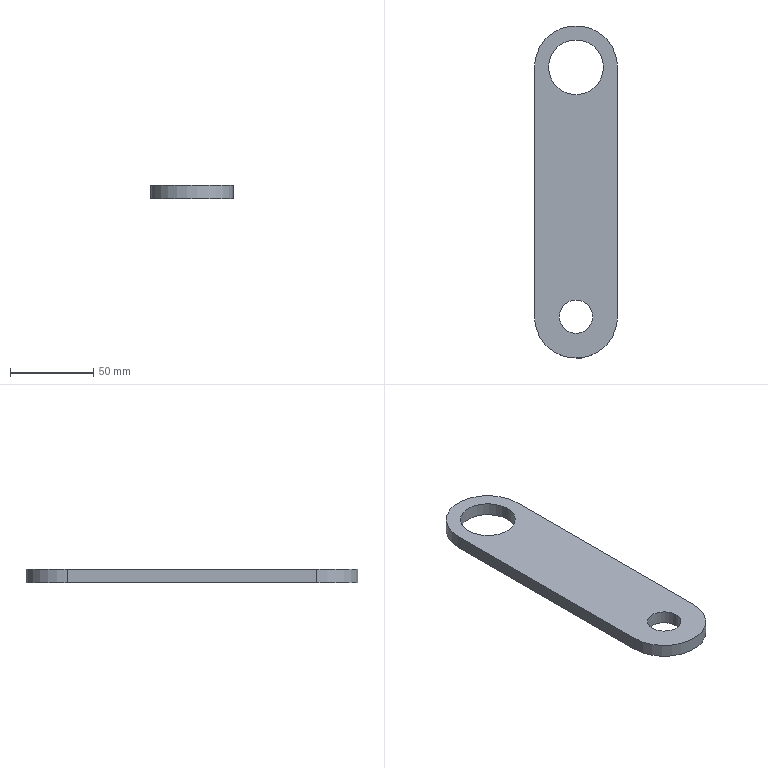Part | STEP file | 1 solid | 10 faces | box 50 x 200 x 8 mm | volume 66352 mm3 | cylinder 6 | plane 4 | commonest cylinder face diameters 20 x2 33 x2 50 x2
STEP:
#1=CARTESIAN_POINT('',(0.,0.,0.));
#2=DIRECTION('',(0.,0.,1.));
#3=DIRECTION('',(1.,0.,0.));
#4=AXIS2_PLACEMENT_3D('',#1,#2,#3);
#5=CARTESIAN_POINT('',(10.,-150.,-4.));
#6=VERTEX_POINT('',#5);
#7=CARTESIAN_POINT('',(-10.,-150.,-4.));
#8=VERTEX_POINT('',#7);
#9=CARTESIAN_POINT('',(0.,-150.,-4.));
#10=DIRECTION('',(0.,0.,1.));
#11=DIRECTION('',(1.,0.,0.));
#12=AXIS2_PLACEMENT_3D('',#9,#10,#11);
#13=CIRCLE('',#12,10.);
#14=CARTESIAN_POINT('',(0.,-150.,4.));
#15=DIRECTION('',(0.,0.,-1.));
#16=DIRECTION('',(-1.,0.,0.));
#17=AXIS2_PLACEMENT_3D('',#14,#15,#16);
#18=CYLINDRICAL_SURFACE('',#17,10.);
#19=CARTESIAN_POINT('',(3.142,8.));
#20=DIRECTION('',(-1.,0.));
#21=VECTOR('',#20,1.);
#22=LINE('',#19,#21);
#23=(GEOMETRIC_REPRESENTATION_CONTEXT(2)PARAMETRIC_REPRESENTATION_CONTEXT()REPRESENTATION_CONTEXT('',''));
#24=DEFINITIONAL_REPRESENTATION('',(#22),#23);
#25=PCURVE('',#18,#24);
#26=CARTESIAN_POINT('',(0.,0.,-4.));
#27=DIRECTION('',(0.,0.,1.));
#28=DIRECTION('',(1.,0.,0.));
#29=AXIS2_PLACEMENT_3D('',#26,#27,#28);
#30=PLANE('',#29);
#31=CARTESIAN_POINT('',(0.,-150.));
#32=DIRECTION('',(1.,0.));
#33=AXIS2_PLACEMENT_2D('',#31,#32);
#34=CIRCLE('',#33,10.);
#35=(GEOMETRIC_REPRESENTATION_CONTEXT(2)PARAMETRIC_REPRESENTATION_CONTEXT()REPRESENTATION_CONTEXT('',''));
#36=DEFINITIONAL_REPRESENTATION('',(#34),#35);
#37=PCURVE('',#30,#36);
#38=SURFACE_CURVE('',#13,(#25,#37),.PCURVE_S1.);
#39=EDGE_CURVE('',#6,#8,#38,.T.);
#40=ORIENTED_EDGE('',*,*,#39,.T.);
#41=CARTESIAN_POINT('',(-10.,-150.,4.));
#42=VERTEX_POINT('',#41);
#43=CARTESIAN_POINT('',(-10.,-150.,4.));
#44=DIRECTION('',(0.,0.,-1.));
#45=VECTOR('',#44,1.);
#46=LINE('',#43,#45);
#47=CARTESIAN_POINT('',(0.,0.));
#48=DIRECTION('',(0.,1.));
#49=VECTOR('',#48,1.);
#50=LINE('',#47,#49);
#51=(GEOMETRIC_REPRESENTATION_CONTEXT(2)PARAMETRIC_REPRESENTATION_CONTEXT()REPRESENTATION_CONTEXT('',''));
#52=DEFINITIONAL_REPRESENTATION('',(#50),#51);
#53=PCURVE('',#18,#52);
#54=CARTESIAN_POINT('',(0.,-150.,4.));
#55=DIRECTION('',(0.,0.,-1.));
#56=DIRECTION('',(-1.,0.,0.));
#57=AXIS2_PLACEMENT_3D('',#54,#55,#56);
#58=CYLINDRICAL_SURFACE('',#57,10.);
#59=CARTESIAN_POINT('',(6.283,0.));
#60=DIRECTION('',(0.,1.));
#61=VECTOR('',#60,1.);
#62=LINE('',#59,#61);
#63=(GEOMETRIC_REPRESENTATION_CONTEXT(2)PARAMETRIC_REPRESENTATION_CONTEXT()REPRESENTATION_CONTEXT('',''));
#64=DEFINITIONAL_REPRESENTATION('',(#62),#63);
#65=PCURVE('',#58,#64);
#66=SURFACE_CURVE('',#46,(#53,#65),.PCURVE_S1.);
#67=EDGE_CURVE('',#42,#8,#66,.T.);
#68=ORIENTED_EDGE('',*,*,#67,.F.);
#69=CARTESIAN_POINT('',(10.,-150.,4.));
#70=VERTEX_POINT('',#69);
#71=CARTESIAN_POINT('',(0.,-150.,4.));
#72=DIRECTION('',(0.,0.,1.));
#73=DIRECTION('',(1.,0.,0.));
#74=AXIS2_PLACEMENT_3D('',#71,#72,#73);
#75=CIRCLE('',#74,10.);
#76=CARTESIAN_POINT('',(3.142,0.));
#77=DIRECTION('',(-1.,0.));
#78=VECTOR('',#77,1.);
#79=LINE('',#76,#78);
#80=(GEOMETRIC_REPRESENTATION_CONTEXT(2)PARAMETRIC_REPRESENTATION_CONTEXT()REPRESENTATION_CONTEXT('',''));
#81=DEFINITIONAL_REPRESENTATION('',(#79),#80);
#82=PCURVE('',#18,#81);
#83=CARTESIAN_POINT('',(0.,0.,4.));
#84=DIRECTION('',(0.,0.,1.));
#85=DIRECTION('',(1.,0.,0.));
#86=AXIS2_PLACEMENT_3D('',#83,#84,#85);
#87=PLANE('',#86);
#88=CARTESIAN_POINT('',(0.,-150.));
#89=DIRECTION('',(1.,0.));
#90=AXIS2_PLACEMENT_2D('',#88,#89);
#91=CIRCLE('',#90,10.);
#92=(GEOMETRIC_REPRESENTATION_CONTEXT(2)PARAMETRIC_REPRESENTATION_CONTEXT()REPRESENTATION_CONTEXT('',''));
#93=DEFINITIONAL_REPRESENTATION('',(#91),#92);
#94=PCURVE('',#87,#93);
#95=SURFACE_CURVE('',#75,(#82,#94),.PCURVE_S1.);
#96=EDGE_CURVE('',#70,#42,#95,.T.);
#97=ORIENTED_EDGE('',*,*,#96,.F.);
#98=CARTESIAN_POINT('',(10.,-150.,4.));
#99=DIRECTION('',(0.,0.,-1.));
#100=VECTOR('',#99,1.);
#101=LINE('',#98,#100);
#102=CARTESIAN_POINT('',(3.142,0.));
#103=DIRECTION('',(0.,1.));
#104=VECTOR('',#103,1.);
#105=LINE('',#102,#104);
#106=(GEOMETRIC_REPRESENTATION_CONTEXT(2)PARAMETRIC_REPRESENTATION_CONTEXT()REPRESENTATION_CONTEXT('',''));
#107=DEFINITIONAL_REPRESENTATION('',(#105),#106);
#108=PCURVE('',#18,#107);
#109=CARTESIAN_POINT('',(3.142,0.));
#110=DIRECTION('',(0.,1.));
#111=VECTOR('',#110,1.);
#112=LINE('',#109,#111);
#113=(GEOMETRIC_REPRESENTATION_CONTEXT(2)PARAMETRIC_REPRESENTATION_CONTEXT()REPRESENTATION_CONTEXT('',''));
#114=DEFINITIONAL_REPRESENTATION('',(#112),#113);
#115=PCURVE('',#58,#114);
#116=SURFACE_CURVE('',#101,(#108,#115),.PCURVE_S1.);
#117=EDGE_CURVE('',#70,#6,#116,.T.);
#118=ORIENTED_EDGE('',*,*,#117,.T.);
#119=EDGE_LOOP('',(#40,#68,#97,#118));
#120=FACE_BOUND('',#119,.F.);
#121=ADVANCED_FACE('',(#120),#18,.F.);
#122=CARTESIAN_POINT('',(16.5,0.,-4.));
#123=VERTEX_POINT('',#122);
#124=CARTESIAN_POINT('',(-16.5,0.,-4.));
#125=VERTEX_POINT('',#124);
#126=CARTESIAN_POINT('',(0.,0.,-4.));
#127=DIRECTION('',(0.,0.,1.));
#128=DIRECTION('',(1.,0.,0.));
#129=AXIS2_PLACEMENT_3D('',#126,#127,#128);
#130=CIRCLE('',#129,16.5);
#131=CARTESIAN_POINT('',(0.,0.,4.));
#132=DIRECTION('',(0.,0.,-1.));
#133=DIRECTION('',(-1.,0.,0.));
#134=AXIS2_PLACEMENT_3D('',#131,#132,#133);
#135=CYLINDRICAL_SURFACE('',#134,16.5);
#136=CARTESIAN_POINT('',(3.142,8.));
#137=DIRECTION('',(-1.,0.));
#138=VECTOR('',#137,1.);
#139=LINE('',#136,#138);
#140=(GEOMETRIC_REPRESENTATION_CONTEXT(2)PARAMETRIC_REPRESENTATION_CONTEXT()REPRESENTATION_CONTEXT('',''));
#141=DEFINITIONAL_REPRESENTATION('',(#139),#140);
#142=PCURVE('',#135,#141);
#143=CARTESIAN_POINT('',(0.,0.));
#144=DIRECTION('',(1.,0.));
#145=AXIS2_PLACEMENT_2D('',#143,#144);
#146=CIRCLE('',#145,16.5);
#147=(GEOMETRIC_REPRESENTATION_CONTEXT(2)PARAMETRIC_REPRESENTATION_CONTEXT()REPRESENTATION_CONTEXT('',''));
#148=DEFINITIONAL_REPRESENTATION('',(#146),#147);
#149=PCURVE('',#30,#148);
#150=SURFACE_CURVE('',#130,(#142,#149),.PCURVE_S1.);
#151=EDGE_CURVE('',#123,#125,#150,.T.);
#152=ORIENTED_EDGE('',*,*,#151,.T.);
#153=CARTESIAN_POINT('',(-16.5,0.,4.));
#154=VERTEX_POINT('',#153);
#155=CARTESIAN_POINT('',(-16.5,0.,4.));
#156=DIRECTION('',(0.,0.,-1.));
#157=VECTOR('',#156,1.);
#158=LINE('',#155,#157);
#159=CARTESIAN_POINT('',(0.,0.));
#160=DIRECTION('',(0.,1.));
#161=VECTOR('',#160,1.);
#162=LINE('',#159,#161);
#163=(GEOMETRIC_REPRESENTATION_CONTEXT(2)PARAMETRIC_REPRESENTATION_CONTEXT()REPRESENTATION_CONTEXT('',''));
#164=DEFINITIONAL_REPRESENTATION('',(#162),#163);
#165=PCURVE('',#135,#164);
#166=CARTESIAN_POINT('',(0.,0.,4.));
#167=DIRECTION('',(0.,0.,-1.));
#168=DIRECTION('',(-1.,0.,0.));
#169=AXIS2_PLACEMENT_3D('',#166,#167,#168);
#170=CYLINDRICAL_SURFACE('',#169,16.5);
#171=CARTESIAN_POINT('',(6.283,0.));
#172=DIRECTION('',(0.,1.));
#173=VECTOR('',#172,1.);
#174=LINE('',#171,#173);
#175=(GEOMETRIC_REPRESENTATION_CONTEXT(2)PARAMETRIC_REPRESENTATION_CONTEXT()REPRESENTATION_CONTEXT('',''));
#176=DEFINITIONAL_REPRESENTATION('',(#174),#175);
#177=PCURVE('',#170,#176);
#178=SURFACE_CURVE('',#158,(#165,#177),.PCURVE_S1.);
#179=EDGE_CURVE('',#154,#125,#178,.T.);
#180=ORIENTED_EDGE('',*,*,#179,.F.);
#181=CARTESIAN_POINT('',(16.5,0.,4.));
#182=VERTEX_POINT('',#181);
#183=CARTESIAN_POINT('',(0.,0.,4.));
#184=DIRECTION('',(0.,0.,1.));
#185=DIRECTION('',(1.,0.,0.));
#186=AXIS2_PLACEMENT_3D('',#183,#184,#185);
#187=CIRCLE('',#186,16.5);
#188=CARTESIAN_POINT('',(3.142,0.));
#189=DIRECTION('',(-1.,0.));
#190=VECTOR('',#189,1.);
#191=LINE('',#188,#190);
#192=(GEOMETRIC_REPRESENTATION_CONTEXT(2)PARAMETRIC_REPRESENTATION_CONTEXT()REPRESENTATION_CONTEXT('',''));
#193=DEFINITIONAL_REPRESENTATION('',(#191),#192);
#194=PCURVE('',#135,#193);
#195=CARTESIAN_POINT('',(0.,0.));
#196=DIRECTION('',(1.,0.));
#197=AXIS2_PLACEMENT_2D('',#195,#196);
#198=CIRCLE('',#197,16.5);
#199=(GEOMETRIC_REPRESENTATION_CONTEXT(2)PARAMETRIC_REPRESENTATION_CONTEXT()REPRESENTATION_CONTEXT('',''));
#200=DEFINITIONAL_REPRESENTATION('',(#198),#199);
#201=PCURVE('',#87,#200);
#202=SURFACE_CURVE('',#187,(#194,#201),.PCURVE_S1.);
#203=EDGE_CURVE('',#182,#154,#202,.T.);
#204=ORIENTED_EDGE('',*,*,#203,.F.);
#205=CARTESIAN_POINT('',(16.5,0.,4.));
#206=DIRECTION('',(0.,0.,-1.));
#207=VECTOR('',#206,1.);
#208=LINE('',#205,#207);
#209=CARTESIAN_POINT('',(3.142,0.));
#210=DIRECTION('',(0.,1.));
#211=VECTOR('',#210,1.);
#212=LINE('',#209,#211);
#213=(GEOMETRIC_REPRESENTATION_CONTEXT(2)PARAMETRIC_REPRESENTATION_CONTEXT()REPRESENTATION_CONTEXT('',''));
#214=DEFINITIONAL_REPRESENTATION('',(#212),#213);
#215=PCURVE('',#135,#214);
#216=CARTESIAN_POINT('',(3.142,0.));
#217=DIRECTION('',(0.,1.));
#218=VECTOR('',#217,1.);
#219=LINE('',#216,#218);
#220=(GEOMETRIC_REPRESENTATION_CONTEXT(2)PARAMETRIC_REPRESENTATION_CONTEXT()REPRESENTATION_CONTEXT('',''));
#221=DEFINITIONAL_REPRESENTATION('',(#219),#220);
#222=PCURVE('',#170,#221);
#223=SURFACE_CURVE('',#208,(#215,#222),.PCURVE_S1.);
#224=EDGE_CURVE('',#182,#123,#223,.T.);
#225=ORIENTED_EDGE('',*,*,#224,.T.);
#226=EDGE_LOOP('',(#152,#180,#204,#225));
#227=FACE_BOUND('',#226,.F.);
#228=ADVANCED_FACE('',(#227),#135,.F.);
#229=CARTESIAN_POINT('',(25.,-150.,-4.));
#230=VERTEX_POINT('',#229);
#231=CARTESIAN_POINT('',(25.,0.,-4.));
#232=VERTEX_POINT('',#231);
#233=CARTESIAN_POINT('',(25.,0.,-4.));
#234=DIRECTION('',(0.,1.,0.));
#235=VECTOR('',#234,1.);
#236=LINE('',#233,#235);
#237=CARTESIAN_POINT('',(25.,0.,4.));
#238=DIRECTION('',(-1.,0.,0.));
#239=DIRECTION('',(0.,1.,0.));
#240=AXIS2_PLACEMENT_3D('',#237,#238,#239);
#241=PLANE('',#240);
#242=CARTESIAN_POINT('',(0.,8.));
#243=DIRECTION('',(1.,0.));
#244=VECTOR('',#243,1.);
#245=LINE('',#242,#244);
#246=(GEOMETRIC_REPRESENTATION_CONTEXT(2)PARAMETRIC_REPRESENTATION_CONTEXT()REPRESENTATION_CONTEXT('',''));
#247=DEFINITIONAL_REPRESENTATION('',(#245),#246);
#248=PCURVE('',#241,#247);
#249=CARTESIAN_POINT('',(25.,0.));
#250=DIRECTION('',(0.,1.));
#251=VECTOR('',#250,1.);
#252=LINE('',#249,#251);
#253=(GEOMETRIC_REPRESENTATION_CONTEXT(2)PARAMETRIC_REPRESENTATION_CONTEXT()REPRESENTATION_CONTEXT('',''));
#254=DEFINITIONAL_REPRESENTATION('',(#252),#253);
#255=PCURVE('',#30,#254);
#256=SURFACE_CURVE('',#236,(#248,#255),.PCURVE_S1.);
#257=EDGE_CURVE('',#230,#232,#256,.T.);
#258=ORIENTED_EDGE('',*,*,#257,.T.);
#259=CARTESIAN_POINT('',(25.,0.,4.));
#260=VERTEX_POINT('',#259);
#261=CARTESIAN_POINT('',(25.,0.,4.));
#262=DIRECTION('',(0.,0.,-1.));
#263=VECTOR('',#262,1.);
#264=LINE('',#261,#263);
#265=CARTESIAN_POINT('',(0.,0.));
#266=DIRECTION('',(0.,1.));
#267=VECTOR('',#266,1.);
#268=LINE('',#265,#267);
#269=(GEOMETRIC_REPRESENTATION_CONTEXT(2)PARAMETRIC_REPRESENTATION_CONTEXT()REPRESENTATION_CONTEXT('',''));
#270=DEFINITIONAL_REPRESENTATION('',(#268),#269);
#271=PCURVE('',#241,#270);
#272=CARTESIAN_POINT('',(0.,0.,4.));
#273=DIRECTION('',(0.,0.,-1.));
#274=DIRECTION('',(-1.,0.,0.));
#275=AXIS2_PLACEMENT_3D('',#272,#273,#274);
#276=CYLINDRICAL_SURFACE('',#275,25.);
#277=CARTESIAN_POINT('',(3.142,0.));
#278=DIRECTION('',(0.,1.));
#279=VECTOR('',#278,1.);
#280=LINE('',#277,#279);
#281=(GEOMETRIC_REPRESENTATION_CONTEXT(2)PARAMETRIC_REPRESENTATION_CONTEXT()REPRESENTATION_CONTEXT('',''));
#282=DEFINITIONAL_REPRESENTATION('',(#280),#281);
#283=PCURVE('',#276,#282);
#284=SURFACE_CURVE('',#264,(#271,#283),.PCURVE_S1.);
#285=EDGE_CURVE('',#260,#232,#284,.T.);
#286=ORIENTED_EDGE('',*,*,#285,.F.);
#287=CARTESIAN_POINT('',(25.,-150.,4.));
#288=VERTEX_POINT('',#287);
#289=CARTESIAN_POINT('',(25.,0.,4.));
#290=DIRECTION('',(0.,1.,0.));
#291=VECTOR('',#290,1.);
#292=LINE('',#289,#291);
#293=CARTESIAN_POINT('',(0.,0.));
#294=DIRECTION('',(1.,0.));
#295=VECTOR('',#294,1.);
#296=LINE('',#293,#295);
#297=(GEOMETRIC_REPRESENTATION_CONTEXT(2)PARAMETRIC_REPRESENTATION_CONTEXT()REPRESENTATION_CONTEXT('',''));
#298=DEFINITIONAL_REPRESENTATION('',(#296),#297);
#299=PCURVE('',#241,#298);
#300=CARTESIAN_POINT('',(25.,0.));
#301=DIRECTION('',(0.,1.));
#302=VECTOR('',#301,1.);
#303=LINE('',#300,#302);
#304=(GEOMETRIC_REPRESENTATION_CONTEXT(2)PARAMETRIC_REPRESENTATION_CONTEXT()REPRESENTATION_CONTEXT('',''));
#305=DEFINITIONAL_REPRESENTATION('',(#303),#304);
#306=PCURVE('',#87,#305);
#307=SURFACE_CURVE('',#292,(#299,#306),.PCURVE_S1.);
#308=EDGE_CURVE('',#288,#260,#307,.T.);
#309=ORIENTED_EDGE('',*,*,#308,.F.);
#310=CARTESIAN_POINT('',(25.,-150.,4.));
#311=DIRECTION('',(0.,0.,-1.));
#312=VECTOR('',#311,1.);
#313=LINE('',#310,#312);
#314=CARTESIAN_POINT('',(-150.,0.));
#315=DIRECTION('',(0.,1.));
#316=VECTOR('',#315,1.);
#317=LINE('',#314,#316);
#318=(GEOMETRIC_REPRESENTATION_CONTEXT(2)PARAMETRIC_REPRESENTATION_CONTEXT()REPRESENTATION_CONTEXT('',''));
#319=DEFINITIONAL_REPRESENTATION('',(#317),#318);
#320=PCURVE('',#241,#319);
#321=CARTESIAN_POINT('',(0.,-150.,4.));
#322=DIRECTION('',(0.,0.,-1.));
#323=DIRECTION('',(-1.,0.,0.));
#324=AXIS2_PLACEMENT_3D('',#321,#322,#323);
#325=CYLINDRICAL_SURFACE('',#324,25.);
#326=CARTESIAN_POINT('',(3.142,0.));
#327=DIRECTION('',(0.,1.));
#328=VECTOR('',#327,1.);
#329=LINE('',#326,#328);
#330=(GEOMETRIC_REPRESENTATION_CONTEXT(2)PARAMETRIC_REPRESENTATION_CONTEXT()REPRESENTATION_CONTEXT('',''));
#331=DEFINITIONAL_REPRESENTATION('',(#329),#330);
#332=PCURVE('',#325,#331);
#333=SURFACE_CURVE('',#313,(#320,#332),.PCURVE_S1.);
#334=EDGE_CURVE('',#288,#230,#333,.T.);
#335=ORIENTED_EDGE('',*,*,#334,.T.);
#336=EDGE_LOOP('',(#258,#286,#309,#335));
#337=FACE_BOUND('',#336,.T.);
#338=ADVANCED_FACE('',(#337),#241,.F.);
#339=CARTESIAN_POINT('',(-25.,-150.,-4.));
#340=VERTEX_POINT('',#339);
#341=CARTESIAN_POINT('',(0.,-150.,-4.));
#342=DIRECTION('',(0.,0.,1.));
#343=DIRECTION('',(1.,0.,0.));
#344=AXIS2_PLACEMENT_3D('',#341,#342,#343);
#345=CIRCLE('',#344,25.);
#346=CARTESIAN_POINT('',(9.425,8.));
#347=DIRECTION('',(-1.,0.));
#348=VECTOR('',#347,1.);
#349=LINE('',#346,#348);
#350=(GEOMETRIC_REPRESENTATION_CONTEXT(2)PARAMETRIC_REPRESENTATION_CONTEXT()REPRESENTATION_CONTEXT('',''));
#351=DEFINITIONAL_REPRESENTATION('',(#349),#350);
#352=PCURVE('',#325,#351);
#353=CARTESIAN_POINT('',(0.,-150.));
#354=DIRECTION('',(1.,0.));
#355=AXIS2_PLACEMENT_2D('',#353,#354);
#356=CIRCLE('',#355,25.);
#357=(GEOMETRIC_REPRESENTATION_CONTEXT(2)PARAMETRIC_REPRESENTATION_CONTEXT()REPRESENTATION_CONTEXT('',''));
#358=DEFINITIONAL_REPRESENTATION('',(#356),#357);
#359=PCURVE('',#30,#358);
#360=SURFACE_CURVE('',#345,(#352,#359),.PCURVE_S1.);
#361=EDGE_CURVE('',#340,#230,#360,.T.);
#362=ORIENTED_EDGE('',*,*,#361,.T.);
#363=ORIENTED_EDGE('',*,*,#334,.F.);
#364=CARTESIAN_POINT('',(-25.,-150.,4.));
#365=VERTEX_POINT('',#364);
#366=CARTESIAN_POINT('',(0.,-150.,4.));
#367=DIRECTION('',(0.,0.,1.));
#368=DIRECTION('',(1.,0.,0.));
#369=AXIS2_PLACEMENT_3D('',#366,#367,#368);
#370=CIRCLE('',#369,25.);
#371=CARTESIAN_POINT('',(9.425,0.));
#372=DIRECTION('',(-1.,0.));
#373=VECTOR('',#372,1.);
#374=LINE('',#371,#373);
#375=(GEOMETRIC_REPRESENTATION_CONTEXT(2)PARAMETRIC_REPRESENTATION_CONTEXT()REPRESENTATION_CONTEXT('',''));
#376=DEFINITIONAL_REPRESENTATION('',(#374),#375);
#377=PCURVE('',#325,#376);
#378=CARTESIAN_POINT('',(0.,-150.));
#379=DIRECTION('',(1.,0.));
#380=AXIS2_PLACEMENT_2D('',#378,#379);
#381=CIRCLE('',#380,25.);
#382=(GEOMETRIC_REPRESENTATION_CONTEXT(2)PARAMETRIC_REPRESENTATION_CONTEXT()REPRESENTATION_CONTEXT('',''));
#383=DEFINITIONAL_REPRESENTATION('',(#381),#382);
#384=PCURVE('',#87,#383);
#385=SURFACE_CURVE('',#370,(#377,#384),.PCURVE_S1.);
#386=EDGE_CURVE('',#365,#288,#385,.T.);
#387=ORIENTED_EDGE('',*,*,#386,.F.);
#388=CARTESIAN_POINT('',(-25.,-150.,4.));
#389=DIRECTION('',(0.,0.,-1.));
#390=VECTOR('',#389,1.);
#391=LINE('',#388,#390);
#392=CARTESIAN_POINT('',(6.283,0.));
#393=DIRECTION('',(0.,1.));
#394=VECTOR('',#393,1.);
#395=LINE('',#392,#394);
#396=(GEOMETRIC_REPRESENTATION_CONTEXT(2)PARAMETRIC_REPRESENTATION_CONTEXT()REPRESENTATION_CONTEXT('',''));
#397=DEFINITIONAL_REPRESENTATION('',(#395),#396);
#398=PCURVE('',#325,#397);
#399=CARTESIAN_POINT('',(-25.,0.,4.));
#400=DIRECTION('',(1.,0.,0.));
#401=DIRECTION('',(0.,1.,0.));
#402=AXIS2_PLACEMENT_3D('',#399,#400,#401);
#403=PLANE('',#402);
#404=CARTESIAN_POINT('',(-150.,0.));
#405=DIRECTION('',(0.,-1.));
#406=VECTOR('',#405,1.);
#407=LINE('',#404,#406);
#408=(GEOMETRIC_REPRESENTATION_CONTEXT(2)PARAMETRIC_REPRESENTATION_CONTEXT()REPRESENTATION_CONTEXT('',''));
#409=DEFINITIONAL_REPRESENTATION('',(#407),#408);
#410=PCURVE('',#403,#409);
#411=SURFACE_CURVE('',#391,(#398,#410),.PCURVE_S1.);
#412=EDGE_CURVE('',#365,#340,#411,.T.);
#413=ORIENTED_EDGE('',*,*,#412,.T.);
#414=EDGE_LOOP('',(#362,#363,#387,#413));
#415=FACE_BOUND('',#414,.T.);
#416=ADVANCED_FACE('',(#415),#325,.T.);
#417=CARTESIAN_POINT('',(-25.,0.,-4.));
#418=VERTEX_POINT('',#417);
#419=CARTESIAN_POINT('',(-25.,0.,-4.));
#420=DIRECTION('',(0.,-1.,0.));
#421=VECTOR('',#420,1.);
#422=LINE('',#419,#421);
#423=CARTESIAN_POINT('',(0.,-8.));
#424=DIRECTION('',(-1.,0.));
#425=VECTOR('',#424,1.);
#426=LINE('',#423,#425);
#427=(GEOMETRIC_REPRESENTATION_CONTEXT(2)PARAMETRIC_REPRESENTATION_CONTEXT()REPRESENTATION_CONTEXT('',''));
#428=DEFINITIONAL_REPRESENTATION('',(#426),#427);
#429=PCURVE('',#403,#428);
#430=CARTESIAN_POINT('',(-25.,0.));
#431=DIRECTION('',(0.,-1.));
#432=VECTOR('',#431,1.);
#433=LINE('',#430,#432);
#434=(GEOMETRIC_REPRESENTATION_CONTEXT(2)PARAMETRIC_REPRESENTATION_CONTEXT()REPRESENTATION_CONTEXT('',''));
#435=DEFINITIONAL_REPRESENTATION('',(#433),#434);
#436=PCURVE('',#30,#435);
#437=SURFACE_CURVE('',#422,(#429,#436),.PCURVE_S1.);
#438=EDGE_CURVE('',#418,#340,#437,.T.);
#439=ORIENTED_EDGE('',*,*,#438,.T.);
#440=ORIENTED_EDGE('',*,*,#412,.F.);
#441=CARTESIAN_POINT('',(-25.,0.,4.));
#442=VERTEX_POINT('',#441);
#443=CARTESIAN_POINT('',(-25.,0.,4.));
#444=DIRECTION('',(0.,-1.,0.));
#445=VECTOR('',#444,1.);
#446=LINE('',#443,#445);
#447=CARTESIAN_POINT('',(0.,0.));
#448=DIRECTION('',(-1.,0.));
#449=VECTOR('',#448,1.);
#450=LINE('',#447,#449);
#451=(GEOMETRIC_REPRESENTATION_CONTEXT(2)PARAMETRIC_REPRESENTATION_CONTEXT()REPRESENTATION_CONTEXT('',''));
#452=DEFINITIONAL_REPRESENTATION('',(#450),#451);
#453=PCURVE('',#403,#452);
#454=CARTESIAN_POINT('',(-25.,0.));
#455=DIRECTION('',(0.,-1.));
#456=VECTOR('',#455,1.);
#457=LINE('',#454,#456);
#458=(GEOMETRIC_REPRESENTATION_CONTEXT(2)PARAMETRIC_REPRESENTATION_CONTEXT()REPRESENTATION_CONTEXT('',''));
#459=DEFINITIONAL_REPRESENTATION('',(#457),#458);
#460=PCURVE('',#87,#459);
#461=SURFACE_CURVE('',#446,(#453,#460),.PCURVE_S1.);
#462=EDGE_CURVE('',#442,#365,#461,.T.);
#463=ORIENTED_EDGE('',*,*,#462,.F.);
#464=CARTESIAN_POINT('',(-25.,0.,4.));
#465=DIRECTION('',(0.,0.,-1.));
#466=VECTOR('',#465,1.);
#467=LINE('',#464,#466);
#468=CARTESIAN_POINT('',(0.,0.));
#469=DIRECTION('',(0.,-1.));
#470=VECTOR('',#469,1.);
#471=LINE('',#468,#470);
#472=(GEOMETRIC_REPRESENTATION_CONTEXT(2)PARAMETRIC_REPRESENTATION_CONTEXT()REPRESENTATION_CONTEXT('',''));
#473=DEFINITIONAL_REPRESENTATION('',(#471),#472);
#474=PCURVE('',#403,#473);
#475=CARTESIAN_POINT('',(0.,0.));
#476=DIRECTION('',(0.,1.));
#477=VECTOR('',#476,1.);
#478=LINE('',#475,#477);
#479=(GEOMETRIC_REPRESENTATION_CONTEXT(2)PARAMETRIC_REPRESENTATION_CONTEXT()REPRESENTATION_CONTEXT('',''));
#480=DEFINITIONAL_REPRESENTATION('',(#478),#479);
#481=PCURVE('',#276,#480);
#482=SURFACE_CURVE('',#467,(#474,#481),.PCURVE_S1.);
#483=EDGE_CURVE('',#442,#418,#482,.T.);
#484=ORIENTED_EDGE('',*,*,#483,.T.);
#485=EDGE_LOOP('',(#439,#440,#463,#484));
#486=FACE_BOUND('',#485,.T.);
#487=ADVANCED_FACE('',(#486),#403,.F.);
#488=CARTESIAN_POINT('',(0.,0.,-4.));
#489=DIRECTION('',(0.,0.,1.));
#490=DIRECTION('',(1.,0.,0.));
#491=AXIS2_PLACEMENT_3D('',#488,#489,#490);
#492=CIRCLE('',#491,25.);
#493=CARTESIAN_POINT('',(3.142,8.));
#494=DIRECTION('',(-1.,0.));
#495=VECTOR('',#494,1.);
#496=LINE('',#493,#495);
#497=(GEOMETRIC_REPRESENTATION_CONTEXT(2)PARAMETRIC_REPRESENTATION_CONTEXT()REPRESENTATION_CONTEXT('',''));
#498=DEFINITIONAL_REPRESENTATION('',(#496),#497);
#499=PCURVE('',#276,#498);
#500=CARTESIAN_POINT('',(0.,0.));
#501=DIRECTION('',(1.,0.));
#502=AXIS2_PLACEMENT_2D('',#500,#501);
#503=CIRCLE('',#502,25.);
#504=(GEOMETRIC_REPRESENTATION_CONTEXT(2)PARAMETRIC_REPRESENTATION_CONTEXT()REPRESENTATION_CONTEXT('',''));
#505=DEFINITIONAL_REPRESENTATION('',(#503),#504);
#506=PCURVE('',#30,#505);
#507=SURFACE_CURVE('',#492,(#499,#506),.PCURVE_S1.);
#508=EDGE_CURVE('',#232,#418,#507,.T.);
#509=ORIENTED_EDGE('',*,*,#508,.T.);
#510=ORIENTED_EDGE('',*,*,#483,.F.);
#511=CARTESIAN_POINT('',(0.,0.,4.));
#512=DIRECTION('',(0.,0.,1.));
#513=DIRECTION('',(1.,0.,0.));
#514=AXIS2_PLACEMENT_3D('',#511,#512,#513);
#515=CIRCLE('',#514,25.);
#516=CARTESIAN_POINT('',(3.142,0.));
#517=DIRECTION('',(-1.,0.));
#518=VECTOR('',#517,1.);
#519=LINE('',#516,#518);
#520=(GEOMETRIC_REPRESENTATION_CONTEXT(2)PARAMETRIC_REPRESENTATION_CONTEXT()REPRESENTATION_CONTEXT('',''));
#521=DEFINITIONAL_REPRESENTATION('',(#519),#520);
#522=PCURVE('',#276,#521);
#523=CARTESIAN_POINT('',(0.,0.));
#524=DIRECTION('',(1.,0.));
#525=AXIS2_PLACEMENT_2D('',#523,#524);
#526=CIRCLE('',#525,25.);
#527=(GEOMETRIC_REPRESENTATION_CONTEXT(2)PARAMETRIC_REPRESENTATION_CONTEXT()REPRESENTATION_CONTEXT('',''));
#528=DEFINITIONAL_REPRESENTATION('',(#526),#527);
#529=PCURVE('',#87,#528);
#530=SURFACE_CURVE('',#515,(#522,#529),.PCURVE_S1.);
#531=EDGE_CURVE('',#260,#442,#530,.T.);
#532=ORIENTED_EDGE('',*,*,#531,.F.);
#533=ORIENTED_EDGE('',*,*,#285,.T.);
#534=EDGE_LOOP('',(#509,#510,#532,#533));
#535=FACE_BOUND('',#534,.T.);
#536=ADVANCED_FACE('',(#535),#276,.T.);
#537=CARTESIAN_POINT('',(0.,-150.,-4.));
#538=DIRECTION('',(0.,0.,1.));
#539=DIRECTION('',(1.,0.,0.));
#540=AXIS2_PLACEMENT_3D('',#537,#538,#539);
#541=CIRCLE('',#540,10.);
#542=CARTESIAN_POINT('',(0.,-150.));
#543=DIRECTION('',(1.,0.));
#544=AXIS2_PLACEMENT_2D('',#542,#543);
#545=CIRCLE('',#544,10.);
#546=(GEOMETRIC_REPRESENTATION_CONTEXT(2)PARAMETRIC_REPRESENTATION_CONTEXT()REPRESENTATION_CONTEXT('',''));
#547=DEFINITIONAL_REPRESENTATION('',(#545),#546);
#548=PCURVE('',#30,#547);
#549=CARTESIAN_POINT('',(9.425,8.));
#550=DIRECTION('',(-1.,0.));
#551=VECTOR('',#550,1.);
#552=LINE('',#549,#551);
#553=(GEOMETRIC_REPRESENTATION_CONTEXT(2)PARAMETRIC_REPRESENTATION_CONTEXT()REPRESENTATION_CONTEXT('',''));
#554=DEFINITIONAL_REPRESENTATION('',(#552),#553);
#555=PCURVE('',#58,#554);
#556=SURFACE_CURVE('',#541,(#548,#555),.PCURVE_S1.);
#557=EDGE_CURVE('',#8,#6,#556,.T.);
#558=ORIENTED_EDGE('',*,*,#557,.T.);
#559=ORIENTED_EDGE('',*,*,#39,.T.);
#560=EDGE_LOOP('',(#558,#559));
#561=FACE_BOUND('',#560,.T.);
#562=CARTESIAN_POINT('',(0.,0.,-4.));
#563=DIRECTION('',(0.,0.,1.));
#564=DIRECTION('',(1.,0.,0.));
#565=AXIS2_PLACEMENT_3D('',#562,#563,#564);
#566=CIRCLE('',#565,16.5);
#567=CARTESIAN_POINT('',(0.,0.));
#568=DIRECTION('',(1.,0.));
#569=AXIS2_PLACEMENT_2D('',#567,#568);
#570=CIRCLE('',#569,16.5);
#571=(GEOMETRIC_REPRESENTATION_CONTEXT(2)PARAMETRIC_REPRESENTATION_CONTEXT()REPRESENTATION_CONTEXT('',''));
#572=DEFINITIONAL_REPRESENTATION('',(#570),#571);
#573=PCURVE('',#30,#572);
#574=CARTESIAN_POINT('',(9.425,8.));
#575=DIRECTION('',(-1.,0.));
#576=VECTOR('',#575,1.);
#577=LINE('',#574,#576);
#578=(GEOMETRIC_REPRESENTATION_CONTEXT(2)PARAMETRIC_REPRESENTATION_CONTEXT()REPRESENTATION_CONTEXT('',''));
#579=DEFINITIONAL_REPRESENTATION('',(#577),#578);
#580=PCURVE('',#170,#579);
#581=SURFACE_CURVE('',#566,(#573,#580),.PCURVE_S1.);
#582=EDGE_CURVE('',#125,#123,#581,.T.);
#583=ORIENTED_EDGE('',*,*,#582,.T.);
#584=ORIENTED_EDGE('',*,*,#151,.T.);
#585=EDGE_LOOP('',(#583,#584));
#586=FACE_BOUND('',#585,.T.);
#587=ORIENTED_EDGE('',*,*,#508,.F.);
#588=ORIENTED_EDGE('',*,*,#257,.F.);
#589=ORIENTED_EDGE('',*,*,#361,.F.);
#590=ORIENTED_EDGE('',*,*,#438,.F.);
#591=EDGE_LOOP('',(#587,#588,#589,#590));
#592=FACE_BOUND('',#591,.T.);
#593=ADVANCED_FACE('',(#561,#586,#592),#30,.F.);
#594=CARTESIAN_POINT('',(0.,-150.,4.));
#595=DIRECTION('',(0.,0.,1.));
#596=DIRECTION('',(1.,0.,0.));
#597=AXIS2_PLACEMENT_3D('',#594,#595,#596);
#598=CIRCLE('',#597,10.);
#599=CARTESIAN_POINT('',(0.,-150.));
#600=DIRECTION('',(1.,0.));
#601=AXIS2_PLACEMENT_2D('',#599,#600);
#602=CIRCLE('',#601,10.);
#603=(GEOMETRIC_REPRESENTATION_CONTEXT(2)PARAMETRIC_REPRESENTATION_CONTEXT()REPRESENTATION_CONTEXT('',''));
#604=DEFINITIONAL_REPRESENTATION('',(#602),#603);
#605=PCURVE('',#87,#604);
#606=CARTESIAN_POINT('',(9.425,0.));
#607=DIRECTION('',(-1.,0.));
#608=VECTOR('',#607,1.);
#609=LINE('',#606,#608);
#610=(GEOMETRIC_REPRESENTATION_CONTEXT(2)PARAMETRIC_REPRESENTATION_CONTEXT()REPRESENTATION_CONTEXT('',''));
#611=DEFINITIONAL_REPRESENTATION('',(#609),#610);
#612=PCURVE('',#58,#611);
#613=SURFACE_CURVE('',#598,(#605,#612),.PCURVE_S1.);
#614=EDGE_CURVE('',#42,#70,#613,.T.);
#615=ORIENTED_EDGE('',*,*,#614,.F.);
#616=ORIENTED_EDGE('',*,*,#96,.F.);
#617=EDGE_LOOP('',(#615,#616));
#618=FACE_BOUND('',#617,.T.);
#619=CARTESIAN_POINT('',(0.,0.,4.));
#620=DIRECTION('',(0.,0.,1.));
#621=DIRECTION('',(1.,0.,0.));
#622=AXIS2_PLACEMENT_3D('',#619,#620,#621);
#623=CIRCLE('',#622,16.5);
#624=CARTESIAN_POINT('',(0.,0.));
#625=DIRECTION('',(1.,0.));
#626=AXIS2_PLACEMENT_2D('',#624,#625);
#627=CIRCLE('',#626,16.5);
#628=(GEOMETRIC_REPRESENTATION_CONTEXT(2)PARAMETRIC_REPRESENTATION_CONTEXT()REPRESENTATION_CONTEXT('',''));
#629=DEFINITIONAL_REPRESENTATION('',(#627),#628);
#630=PCURVE('',#87,#629);
#631=CARTESIAN_POINT('',(9.425,0.));
#632=DIRECTION('',(-1.,0.));
#633=VECTOR('',#632,1.);
#634=LINE('',#631,#633);
#635=(GEOMETRIC_REPRESENTATION_CONTEXT(2)PARAMETRIC_REPRESENTATION_CONTEXT()REPRESENTATION_CONTEXT('',''));
#636=DEFINITIONAL_REPRESENTATION('',(#634),#635);
#637=PCURVE('',#170,#636);
#638=SURFACE_CURVE('',#623,(#630,#637),.PCURVE_S1.);
#639=EDGE_CURVE('',#154,#182,#638,.T.);
#640=ORIENTED_EDGE('',*,*,#639,.F.);
#641=ORIENTED_EDGE('',*,*,#203,.F.);
#642=EDGE_LOOP('',(#640,#641));
#643=FACE_BOUND('',#642,.T.);
#644=ORIENTED_EDGE('',*,*,#531,.T.);
#645=ORIENTED_EDGE('',*,*,#462,.T.);
#646=ORIENTED_EDGE('',*,*,#386,.T.);
#647=ORIENTED_EDGE('',*,*,#308,.T.);
#648=EDGE_LOOP('',(#644,#645,#646,#647));
#649=FACE_BOUND('',#648,.T.);
#650=ADVANCED_FACE('',(#618,#643,#649),#87,.T.);
#651=ORIENTED_EDGE('',*,*,#179,.T.);
#652=ORIENTED_EDGE('',*,*,#582,.T.);
#653=ORIENTED_EDGE('',*,*,#224,.F.);
#654=ORIENTED_EDGE('',*,*,#639,.F.);
#655=EDGE_LOOP('',(#651,#652,#653,#654));
#656=FACE_BOUND('',#655,.F.);
#657=ADVANCED_FACE('',(#656),#170,.F.);
#658=ORIENTED_EDGE('',*,*,#67,.T.);
#659=ORIENTED_EDGE('',*,*,#557,.T.);
#660=ORIENTED_EDGE('',*,*,#117,.F.);
#661=ORIENTED_EDGE('',*,*,#614,.F.);
#662=EDGE_LOOP('',(#658,#659,#660,#661));
#663=FACE_BOUND('',#662,.F.);
#664=ADVANCED_FACE('',(#663),#58,.F.);
#665=CLOSED_SHELL('',(#121,#228,#338,#416,#487,#536,#593,#650,#657,#664));
#666=MANIFOLD_SOLID_BREP('',#665);
#667=(LENGTH_UNIT()NAMED_UNIT(*)SI_UNIT(.MILLI.,.METRE.));
#668=UNCERTAINTY_MEASURE_WITH_UNIT(LENGTH_MEASURE(0.0000001),#667,'','');
#669=(NAMED_UNIT(*)PLANE_ANGLE_UNIT()SI_UNIT($,.RADIAN.));
#670=(NAMED_UNIT(*)SI_UNIT($,.STERADIAN.)SOLID_ANGLE_UNIT());
#671=(GEOMETRIC_REPRESENTATION_CONTEXT(3)GLOBAL_UNCERTAINTY_ASSIGNED_CONTEXT((#668))GLOBAL_UNIT_ASSIGNED_CONTEXT((#667,#669,#670))REPRESENTATION_CONTEXT('',''));
#672=ADVANCED_BREP_SHAPE_REPRESENTATION('',(#4,#666),#671);